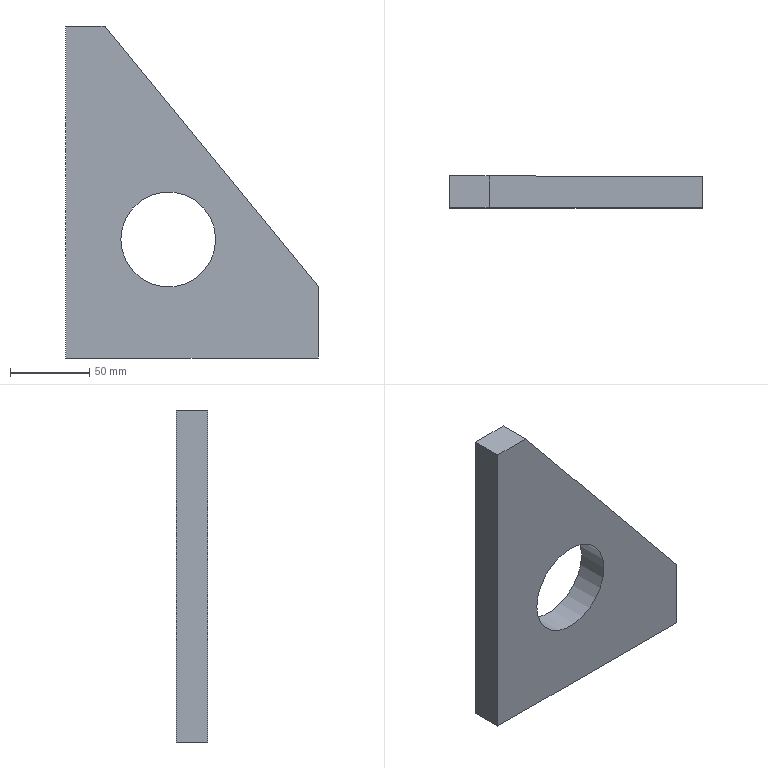Part | STEP file | Tube necking machine_id558_x_t | 1 solid | 8 faces | box 160 x 20 x 210 mm | volume 392701 mm3 | plane 7 | cylinder 1 | commonest cylinder face diameters 60 x1
STEP:
#1=CARTESIAN_POINT('',(0.,0.,0.));
#2=DIRECTION('',(0.,0.,1.));
#3=DIRECTION('',(1.,0.,0.));
#4=AXIS2_PLACEMENT_3D('',#1,#2,#3);
#5=CARTESIAN_POINT('',(387.5,115.,20.));
#6=VERTEX_POINT('',#5);
#7=CARTESIAN_POINT('',(387.5,115.,230.));
#8=VERTEX_POINT('',#7);
#9=CARTESIAN_POINT('',(387.5,115.,230.));
#10=DIRECTION('',(0.,0.,1.));
#11=VECTOR('',#10,1.);
#12=LINE('',#9,#11);
#13=CARTESIAN_POINT('',(387.5,95.,230.));
#14=DIRECTION('',(-1.,0.,0.));
#15=DIRECTION('',(0.,0.,1.));
#16=AXIS2_PLACEMENT_3D('',#13,#14,#15);
#17=PLANE('',#16);
#18=CARTESIAN_POINT('',(0.,20.));
#19=DIRECTION('',(1.,0.));
#20=VECTOR('',#19,1.);
#21=LINE('',#18,#20);
#22=(GEOMETRIC_REPRESENTATION_CONTEXT(2)PARAMETRIC_REPRESENTATION_CONTEXT()REPRESENTATION_CONTEXT('',''));
#23=DEFINITIONAL_REPRESENTATION('',(#21),#22);
#24=PCURVE('',#17,#23);
#25=CARTESIAN_POINT('',(452.5,115.,95.));
#26=DIRECTION('',(0.,1.,0.));
#27=DIRECTION('',(0.,0.,-1.));
#28=AXIS2_PLACEMENT_3D('',#25,#26,#27);
#29=PLANE('',#28);
#30=CARTESIAN_POINT('',(-135.,65.));
#31=DIRECTION('',(-1.,0.));
#32=VECTOR('',#31,1.);
#33=LINE('',#30,#32);
#34=(GEOMETRIC_REPRESENTATION_CONTEXT(2)PARAMETRIC_REPRESENTATION_CONTEXT()REPRESENTATION_CONTEXT('',''));
#35=DEFINITIONAL_REPRESENTATION('',(#33),#34);
#36=PCURVE('',#29,#35);
#37=SURFACE_CURVE('',#12,(#24,#36),.PCURVE_S1.);
#38=EDGE_CURVE('',#6,#8,#37,.T.);
#39=ORIENTED_EDGE('',*,*,#38,.F.);
#40=CARTESIAN_POINT('',(387.5,95.,20.));
#41=VERTEX_POINT('',#40);
#42=CARTESIAN_POINT('',(387.5,95.,20.));
#43=DIRECTION('',(0.,-1.,0.));
#44=VECTOR('',#43,1.);
#45=LINE('',#42,#44);
#46=CARTESIAN_POINT('',(-210.,0.));
#47=DIRECTION('',(0.,-1.));
#48=VECTOR('',#47,1.);
#49=LINE('',#46,#48);
#50=(GEOMETRIC_REPRESENTATION_CONTEXT(2)PARAMETRIC_REPRESENTATION_CONTEXT()REPRESENTATION_CONTEXT('',''));
#51=DEFINITIONAL_REPRESENTATION('',(#49),#50);
#52=PCURVE('',#17,#51);
#53=CARTESIAN_POINT('',(387.5,95.,20.));
#54=DIRECTION('',(0.,0.,-1.));
#55=DIRECTION('',(-1.,0.,0.));
#56=AXIS2_PLACEMENT_3D('',#53,#54,#55);
#57=PLANE('',#56);
#58=CARTESIAN_POINT('',(0.,0.));
#59=DIRECTION('',(0.,-1.));
#60=VECTOR('',#59,1.);
#61=LINE('',#58,#60);
#62=(GEOMETRIC_REPRESENTATION_CONTEXT(2)PARAMETRIC_REPRESENTATION_CONTEXT()REPRESENTATION_CONTEXT('',''));
#63=DEFINITIONAL_REPRESENTATION('',(#61),#62);
#64=PCURVE('',#57,#63);
#65=SURFACE_CURVE('',#45,(#52,#64),.PCURVE_S1.);
#66=EDGE_CURVE('',#6,#41,#65,.T.);
#67=ORIENTED_EDGE('',*,*,#66,.T.);
#68=CARTESIAN_POINT('',(387.5,95.,230.));
#69=VERTEX_POINT('',#68);
#70=CARTESIAN_POINT('',(387.5,95.,230.));
#71=DIRECTION('',(0.,0.,1.));
#72=VECTOR('',#71,1.);
#73=LINE('',#70,#72);
#74=CARTESIAN_POINT('',(0.,0.));
#75=DIRECTION('',(1.,0.));
#76=VECTOR('',#75,1.);
#77=LINE('',#74,#76);
#78=(GEOMETRIC_REPRESENTATION_CONTEXT(2)PARAMETRIC_REPRESENTATION_CONTEXT()REPRESENTATION_CONTEXT('',''));
#79=DEFINITIONAL_REPRESENTATION('',(#77),#78);
#80=PCURVE('',#17,#79);
#81=CARTESIAN_POINT('',(452.5,95.,95.));
#82=DIRECTION('',(0.,1.,0.));
#83=DIRECTION('',(0.,0.,-1.));
#84=AXIS2_PLACEMENT_3D('',#81,#82,#83);
#85=PLANE('',#84);
#86=CARTESIAN_POINT('',(-135.,65.));
#87=DIRECTION('',(-1.,0.));
#88=VECTOR('',#87,1.);
#89=LINE('',#86,#88);
#90=(GEOMETRIC_REPRESENTATION_CONTEXT(2)PARAMETRIC_REPRESENTATION_CONTEXT()REPRESENTATION_CONTEXT('',''));
#91=DEFINITIONAL_REPRESENTATION('',(#89),#90);
#92=PCURVE('',#85,#91);
#93=SURFACE_CURVE('',#73,(#80,#92),.PCURVE_S1.);
#94=EDGE_CURVE('',#41,#69,#93,.T.);
#95=ORIENTED_EDGE('',*,*,#94,.T.);
#96=CARTESIAN_POINT('',(387.5,95.,230.));
#97=DIRECTION('',(0.,-1.,0.));
#98=VECTOR('',#97,1.);
#99=LINE('',#96,#98);
#100=CARTESIAN_POINT('',(0.,0.));
#101=DIRECTION('',(0.,-1.));
#102=VECTOR('',#101,1.);
#103=LINE('',#100,#102);
#104=(GEOMETRIC_REPRESENTATION_CONTEXT(2)PARAMETRIC_REPRESENTATION_CONTEXT()REPRESENTATION_CONTEXT('',''));
#105=DEFINITIONAL_REPRESENTATION('',(#103),#104);
#106=PCURVE('',#17,#105);
#107=CARTESIAN_POINT('',(412.5,95.,230.));
#108=DIRECTION('',(0.,0.,1.));
#109=DIRECTION('',(1.,0.,0.));
#110=AXIS2_PLACEMENT_3D('',#107,#108,#109);
#111=PLANE('',#110);
#112=CARTESIAN_POINT('',(-25.,0.));
#113=DIRECTION('',(0.,-1.));
#114=VECTOR('',#113,1.);
#115=LINE('',#112,#114);
#116=(GEOMETRIC_REPRESENTATION_CONTEXT(2)PARAMETRIC_REPRESENTATION_CONTEXT()REPRESENTATION_CONTEXT('',''));
#117=DEFINITIONAL_REPRESENTATION('',(#115),#116);
#118=PCURVE('',#111,#117);
#119=SURFACE_CURVE('',#99,(#106,#118),.PCURVE_S1.);
#120=EDGE_CURVE('',#8,#69,#119,.T.);
#121=ORIENTED_EDGE('',*,*,#120,.F.);
#122=EDGE_LOOP('',(#39,#67,#95,#121));
#123=FACE_BOUND('',#122,.T.);
#124=ADVANCED_FACE('',(#123),#17,.T.);
#125=CARTESIAN_POINT('',(547.5,115.,20.));
#126=VERTEX_POINT('',#125);
#127=CARTESIAN_POINT('',(387.5,115.,20.));
#128=DIRECTION('',(-1.,0.,0.));
#129=VECTOR('',#128,1.);
#130=LINE('',#127,#129);
#131=CARTESIAN_POINT('',(0.,20.));
#132=DIRECTION('',(1.,0.));
#133=VECTOR('',#132,1.);
#134=LINE('',#131,#133);
#135=(GEOMETRIC_REPRESENTATION_CONTEXT(2)PARAMETRIC_REPRESENTATION_CONTEXT()REPRESENTATION_CONTEXT('',''));
#136=DEFINITIONAL_REPRESENTATION('',(#134),#135);
#137=PCURVE('',#57,#136);
#138=CARTESIAN_POINT('',(75.,65.));
#139=DIRECTION('',(0.,1.));
#140=VECTOR('',#139,1.);
#141=LINE('',#138,#140);
#142=(GEOMETRIC_REPRESENTATION_CONTEXT(2)PARAMETRIC_REPRESENTATION_CONTEXT()REPRESENTATION_CONTEXT('',''));
#143=DEFINITIONAL_REPRESENTATION('',(#141),#142);
#144=PCURVE('',#29,#143);
#145=SURFACE_CURVE('',#130,(#137,#144),.PCURVE_S1.);
#146=EDGE_CURVE('',#126,#6,#145,.T.);
#147=ORIENTED_EDGE('',*,*,#146,.F.);
#148=CARTESIAN_POINT('',(547.5,95.,20.));
#149=VERTEX_POINT('',#148);
#150=CARTESIAN_POINT('',(547.5,95.,20.));
#151=DIRECTION('',(0.,-1.,0.));
#152=VECTOR('',#151,1.);
#153=LINE('',#150,#152);
#154=CARTESIAN_POINT('',(-160.,0.));
#155=DIRECTION('',(0.,-1.));
#156=VECTOR('',#155,1.);
#157=LINE('',#154,#156);
#158=(GEOMETRIC_REPRESENTATION_CONTEXT(2)PARAMETRIC_REPRESENTATION_CONTEXT()REPRESENTATION_CONTEXT('',''));
#159=DEFINITIONAL_REPRESENTATION('',(#157),#158);
#160=PCURVE('',#57,#159);
#161=CARTESIAN_POINT('',(547.5,95.,20.));
#162=DIRECTION('',(1.,0.,0.));
#163=DIRECTION('',(0.,0.,-1.));
#164=AXIS2_PLACEMENT_3D('',#161,#162,#163);
#165=PLANE('',#164);
#166=CARTESIAN_POINT('',(0.,0.));
#167=DIRECTION('',(0.,-1.));
#168=VECTOR('',#167,1.);
#169=LINE('',#166,#168);
#170=(GEOMETRIC_REPRESENTATION_CONTEXT(2)PARAMETRIC_REPRESENTATION_CONTEXT()REPRESENTATION_CONTEXT('',''));
#171=DEFINITIONAL_REPRESENTATION('',(#169),#170);
#172=PCURVE('',#165,#171);
#173=SURFACE_CURVE('',#153,(#160,#172),.PCURVE_S1.);
#174=EDGE_CURVE('',#126,#149,#173,.T.);
#175=ORIENTED_EDGE('',*,*,#174,.T.);
#176=CARTESIAN_POINT('',(387.5,95.,20.));
#177=DIRECTION('',(-1.,0.,0.));
#178=VECTOR('',#177,1.);
#179=LINE('',#176,#178);
#180=CARTESIAN_POINT('',(0.,0.));
#181=DIRECTION('',(1.,0.));
#182=VECTOR('',#181,1.);
#183=LINE('',#180,#182);
#184=(GEOMETRIC_REPRESENTATION_CONTEXT(2)PARAMETRIC_REPRESENTATION_CONTEXT()REPRESENTATION_CONTEXT('',''));
#185=DEFINITIONAL_REPRESENTATION('',(#183),#184);
#186=PCURVE('',#57,#185);
#187=CARTESIAN_POINT('',(75.,65.));
#188=DIRECTION('',(0.,1.));
#189=VECTOR('',#188,1.);
#190=LINE('',#187,#189);
#191=(GEOMETRIC_REPRESENTATION_CONTEXT(2)PARAMETRIC_REPRESENTATION_CONTEXT()REPRESENTATION_CONTEXT('',''));
#192=DEFINITIONAL_REPRESENTATION('',(#190),#191);
#193=PCURVE('',#85,#192);
#194=SURFACE_CURVE('',#179,(#186,#193),.PCURVE_S1.);
#195=EDGE_CURVE('',#149,#41,#194,.T.);
#196=ORIENTED_EDGE('',*,*,#195,.T.);
#197=ORIENTED_EDGE('',*,*,#66,.F.);
#198=EDGE_LOOP('',(#147,#175,#196,#197));
#199=FACE_BOUND('',#198,.T.);
#200=ADVANCED_FACE('',(#199),#57,.T.);
#201=CARTESIAN_POINT('',(547.5,115.,65.));
#202=VERTEX_POINT('',#201);
#203=CARTESIAN_POINT('',(547.5,115.,20.));
#204=DIRECTION('',(0.,0.,-1.));
#205=VECTOR('',#204,1.);
#206=LINE('',#203,#205);
#207=CARTESIAN_POINT('',(0.,20.));
#208=DIRECTION('',(1.,0.));
#209=VECTOR('',#208,1.);
#210=LINE('',#207,#209);
#211=(GEOMETRIC_REPRESENTATION_CONTEXT(2)PARAMETRIC_REPRESENTATION_CONTEXT()REPRESENTATION_CONTEXT('',''));
#212=DEFINITIONAL_REPRESENTATION('',(#210),#211);
#213=PCURVE('',#165,#212);
#214=CARTESIAN_POINT('',(75.,-95.));
#215=DIRECTION('',(1.,0.));
#216=VECTOR('',#215,1.);
#217=LINE('',#214,#216);
#218=(GEOMETRIC_REPRESENTATION_CONTEXT(2)PARAMETRIC_REPRESENTATION_CONTEXT()REPRESENTATION_CONTEXT('',''));
#219=DEFINITIONAL_REPRESENTATION('',(#217),#218);
#220=PCURVE('',#29,#219);
#221=SURFACE_CURVE('',#206,(#213,#220),.PCURVE_S1.);
#222=EDGE_CURVE('',#202,#126,#221,.T.);
#223=ORIENTED_EDGE('',*,*,#222,.F.);
#224=CARTESIAN_POINT('',(547.5,95.,65.));
#225=VERTEX_POINT('',#224);
#226=CARTESIAN_POINT('',(547.5,95.,65.));
#227=DIRECTION('',(0.,-1.,0.));
#228=VECTOR('',#227,1.);
#229=LINE('',#226,#228);
#230=CARTESIAN_POINT('',(-45.,0.));
#231=DIRECTION('',(0.,-1.));
#232=VECTOR('',#231,1.);
#233=LINE('',#230,#232);
#234=(GEOMETRIC_REPRESENTATION_CONTEXT(2)PARAMETRIC_REPRESENTATION_CONTEXT()REPRESENTATION_CONTEXT('',''));
#235=DEFINITIONAL_REPRESENTATION('',(#233),#234);
#236=PCURVE('',#165,#235);
#237=CARTESIAN_POINT('',(547.5,95.,65.));
#238=DIRECTION('',(0.774,0.,0.6332));
#239=DIRECTION('',(0.6332,0.,-0.774));
#240=AXIS2_PLACEMENT_3D('',#237,#238,#239);
#241=PLANE('',#240);
#242=CARTESIAN_POINT('',(0.,0.));
#243=DIRECTION('',(0.,-1.));
#244=VECTOR('',#243,1.);
#245=LINE('',#242,#244);
#246=(GEOMETRIC_REPRESENTATION_CONTEXT(2)PARAMETRIC_REPRESENTATION_CONTEXT()REPRESENTATION_CONTEXT('',''));
#247=DEFINITIONAL_REPRESENTATION('',(#245),#246);
#248=PCURVE('',#241,#247);
#249=SURFACE_CURVE('',#229,(#236,#248),.PCURVE_S1.);
#250=EDGE_CURVE('',#202,#225,#249,.T.);
#251=ORIENTED_EDGE('',*,*,#250,.T.);
#252=CARTESIAN_POINT('',(547.5,95.,20.));
#253=DIRECTION('',(0.,0.,-1.));
#254=VECTOR('',#253,1.);
#255=LINE('',#252,#254);
#256=CARTESIAN_POINT('',(0.,0.));
#257=DIRECTION('',(1.,0.));
#258=VECTOR('',#257,1.);
#259=LINE('',#256,#258);
#260=(GEOMETRIC_REPRESENTATION_CONTEXT(2)PARAMETRIC_REPRESENTATION_CONTEXT()REPRESENTATION_CONTEXT('',''));
#261=DEFINITIONAL_REPRESENTATION('',(#259),#260);
#262=PCURVE('',#165,#261);
#263=CARTESIAN_POINT('',(75.,-95.));
#264=DIRECTION('',(1.,0.));
#265=VECTOR('',#264,1.);
#266=LINE('',#263,#265);
#267=(GEOMETRIC_REPRESENTATION_CONTEXT(2)PARAMETRIC_REPRESENTATION_CONTEXT()REPRESENTATION_CONTEXT('',''));
#268=DEFINITIONAL_REPRESENTATION('',(#266),#267);
#269=PCURVE('',#85,#268);
#270=SURFACE_CURVE('',#255,(#262,#269),.PCURVE_S1.);
#271=EDGE_CURVE('',#225,#149,#270,.T.);
#272=ORIENTED_EDGE('',*,*,#271,.T.);
#273=ORIENTED_EDGE('',*,*,#174,.F.);
#274=EDGE_LOOP('',(#223,#251,#272,#273));
#275=FACE_BOUND('',#274,.T.);
#276=ADVANCED_FACE('',(#275),#165,.T.);
#277=CARTESIAN_POINT('',(412.5,115.,230.));
#278=VERTEX_POINT('',#277);
#279=CARTESIAN_POINT('',(547.5,115.,65.));
#280=DIRECTION('',(0.6332,0.,-0.774));
#281=VECTOR('',#280,1.);
#282=LINE('',#279,#281);
#283=CARTESIAN_POINT('',(0.,20.));
#284=DIRECTION('',(1.,0.));
#285=VECTOR('',#284,1.);
#286=LINE('',#283,#285);
#287=(GEOMETRIC_REPRESENTATION_CONTEXT(2)PARAMETRIC_REPRESENTATION_CONTEXT()REPRESENTATION_CONTEXT('',''));
#288=DEFINITIONAL_REPRESENTATION('',(#286),#287);
#289=PCURVE('',#241,#288);
#290=CARTESIAN_POINT('',(30.,-95.));
#291=DIRECTION('',(0.774,-0.6332));
#292=VECTOR('',#291,1.);
#293=LINE('',#290,#292);
#294=(GEOMETRIC_REPRESENTATION_CONTEXT(2)PARAMETRIC_REPRESENTATION_CONTEXT()REPRESENTATION_CONTEXT('',''));
#295=DEFINITIONAL_REPRESENTATION('',(#293),#294);
#296=PCURVE('',#29,#295);
#297=SURFACE_CURVE('',#282,(#289,#296),.PCURVE_S1.);
#298=EDGE_CURVE('',#278,#202,#297,.T.);
#299=ORIENTED_EDGE('',*,*,#298,.F.);
#300=CARTESIAN_POINT('',(412.5,95.,230.));
#301=VERTEX_POINT('',#300);
#302=CARTESIAN_POINT('',(412.5,95.,230.));
#303=DIRECTION('',(0.,-1.,0.));
#304=VECTOR('',#303,1.);
#305=LINE('',#302,#304);
#306=CARTESIAN_POINT('',(-213.19,0.));
#307=DIRECTION('',(0.,-1.));
#308=VECTOR('',#307,1.);
#309=LINE('',#306,#308);
#310=(GEOMETRIC_REPRESENTATION_CONTEXT(2)PARAMETRIC_REPRESENTATION_CONTEXT()REPRESENTATION_CONTEXT('',''));
#311=DEFINITIONAL_REPRESENTATION('',(#309),#310);
#312=PCURVE('',#241,#311);
#313=CARTESIAN_POINT('',(0.,0.));
#314=DIRECTION('',(0.,-1.));
#315=VECTOR('',#314,1.);
#316=LINE('',#313,#315);
#317=(GEOMETRIC_REPRESENTATION_CONTEXT(2)PARAMETRIC_REPRESENTATION_CONTEXT()REPRESENTATION_CONTEXT('',''));
#318=DEFINITIONAL_REPRESENTATION('',(#316),#317);
#319=PCURVE('',#111,#318);
#320=SURFACE_CURVE('',#305,(#312,#319),.PCURVE_S1.);
#321=EDGE_CURVE('',#278,#301,#320,.T.);
#322=ORIENTED_EDGE('',*,*,#321,.T.);
#323=CARTESIAN_POINT('',(547.5,95.,65.));
#324=DIRECTION('',(0.6332,0.,-0.774));
#325=VECTOR('',#324,1.);
#326=LINE('',#323,#325);
#327=CARTESIAN_POINT('',(0.,0.));
#328=DIRECTION('',(1.,0.));
#329=VECTOR('',#328,1.);
#330=LINE('',#327,#329);
#331=(GEOMETRIC_REPRESENTATION_CONTEXT(2)PARAMETRIC_REPRESENTATION_CONTEXT()REPRESENTATION_CONTEXT('',''));
#332=DEFINITIONAL_REPRESENTATION('',(#330),#331);
#333=PCURVE('',#241,#332);
#334=CARTESIAN_POINT('',(30.,-95.));
#335=DIRECTION('',(0.774,-0.6332));
#336=VECTOR('',#335,1.);
#337=LINE('',#334,#336);
#338=(GEOMETRIC_REPRESENTATION_CONTEXT(2)PARAMETRIC_REPRESENTATION_CONTEXT()REPRESENTATION_CONTEXT('',''));
#339=DEFINITIONAL_REPRESENTATION('',(#337),#338);
#340=PCURVE('',#85,#339);
#341=SURFACE_CURVE('',#326,(#333,#340),.PCURVE_S1.);
#342=EDGE_CURVE('',#301,#225,#341,.T.);
#343=ORIENTED_EDGE('',*,*,#342,.T.);
#344=ORIENTED_EDGE('',*,*,#250,.F.);
#345=EDGE_LOOP('',(#299,#322,#343,#344));
#346=FACE_BOUND('',#345,.T.);
#347=ADVANCED_FACE('',(#346),#241,.T.);
#348=CARTESIAN_POINT('',(412.5,115.,230.));
#349=DIRECTION('',(1.,0.,0.));
#350=VECTOR('',#349,1.);
#351=LINE('',#348,#350);
#352=CARTESIAN_POINT('',(0.,20.));
#353=DIRECTION('',(1.,0.));
#354=VECTOR('',#353,1.);
#355=LINE('',#352,#354);
#356=(GEOMETRIC_REPRESENTATION_CONTEXT(2)PARAMETRIC_REPRESENTATION_CONTEXT()REPRESENTATION_CONTEXT('',''));
#357=DEFINITIONAL_REPRESENTATION('',(#355),#356);
#358=PCURVE('',#111,#357);
#359=CARTESIAN_POINT('',(-135.,40.));
#360=DIRECTION('',(0.,-1.));
#361=VECTOR('',#360,1.);
#362=LINE('',#359,#361);
#363=(GEOMETRIC_REPRESENTATION_CONTEXT(2)PARAMETRIC_REPRESENTATION_CONTEXT()REPRESENTATION_CONTEXT('',''));
#364=DEFINITIONAL_REPRESENTATION('',(#362),#363);
#365=PCURVE('',#29,#364);
#366=SURFACE_CURVE('',#351,(#358,#365),.PCURVE_S1.);
#367=EDGE_CURVE('',#8,#278,#366,.T.);
#368=ORIENTED_EDGE('',*,*,#367,.F.);
#369=ORIENTED_EDGE('',*,*,#120,.T.);
#370=CARTESIAN_POINT('',(412.5,95.,230.));
#371=DIRECTION('',(1.,0.,0.));
#372=VECTOR('',#371,1.);
#373=LINE('',#370,#372);
#374=CARTESIAN_POINT('',(0.,0.));
#375=DIRECTION('',(1.,0.));
#376=VECTOR('',#375,1.);
#377=LINE('',#374,#376);
#378=(GEOMETRIC_REPRESENTATION_CONTEXT(2)PARAMETRIC_REPRESENTATION_CONTEXT()REPRESENTATION_CONTEXT('',''));
#379=DEFINITIONAL_REPRESENTATION('',(#377),#378);
#380=PCURVE('',#111,#379);
#381=CARTESIAN_POINT('',(-135.,40.));
#382=DIRECTION('',(0.,-1.));
#383=VECTOR('',#382,1.);
#384=LINE('',#381,#383);
#385=(GEOMETRIC_REPRESENTATION_CONTEXT(2)PARAMETRIC_REPRESENTATION_CONTEXT()REPRESENTATION_CONTEXT('',''));
#386=DEFINITIONAL_REPRESENTATION('',(#384),#385);
#387=PCURVE('',#85,#386);
#388=SURFACE_CURVE('',#373,(#380,#387),.PCURVE_S1.);
#389=EDGE_CURVE('',#69,#301,#388,.T.);
#390=ORIENTED_EDGE('',*,*,#389,.T.);
#391=ORIENTED_EDGE('',*,*,#321,.F.);
#392=EDGE_LOOP('',(#368,#369,#390,#391));
#393=FACE_BOUND('',#392,.T.);
#394=ADVANCED_FACE('',(#393),#111,.T.);
#395=CARTESIAN_POINT('',(482.5,95.,95.));
#396=VERTEX_POINT('',#395);
#397=CARTESIAN_POINT('',(452.5,95.,95.));
#398=DIRECTION('',(0.,1.,0.));
#399=DIRECTION('',(1.,0.,0.));
#400=AXIS2_PLACEMENT_3D('',#397,#398,#399);
#401=CIRCLE('',#400,30.);
#402=CARTESIAN_POINT('',(452.5,95.,95.));
#403=DIRECTION('',(0.,1.,0.));
#404=DIRECTION('',(0.,0.,-1.));
#405=AXIS2_PLACEMENT_3D('',#402,#403,#404);
#406=CYLINDRICAL_SURFACE('',#405,30.);
#407=CARTESIAN_POINT('',(4.712,0.));
#408=DIRECTION('',(1.,0.));
#409=VECTOR('',#408,1.);
#410=LINE('',#407,#409);
#411=(GEOMETRIC_REPRESENTATION_CONTEXT(2)PARAMETRIC_REPRESENTATION_CONTEXT()REPRESENTATION_CONTEXT('',''));
#412=DEFINITIONAL_REPRESENTATION('',(#410),#411);
#413=PCURVE('',#406,#412);
#414=CARTESIAN_POINT('',(0.,0.));
#415=DIRECTION('',(0.,-1.));
#416=AXIS2_PLACEMENT_2D('',#414,#415);
#417=CIRCLE('',#416,30.);
#418=(GEOMETRIC_REPRESENTATION_CONTEXT(2)PARAMETRIC_REPRESENTATION_CONTEXT()REPRESENTATION_CONTEXT('',''));
#419=DEFINITIONAL_REPRESENTATION('',(#417),#418);
#420=PCURVE('',#85,#419);
#421=SURFACE_CURVE('',#401,(#413,#420),.PCURVE_S1.);
#422=EDGE_CURVE('',#396,#396,#421,.T.);
#423=ORIENTED_EDGE('',*,*,#422,.T.);
#424=CARTESIAN_POINT('',(482.5,115.,95.));
#425=VERTEX_POINT('',#424);
#426=CARTESIAN_POINT('',(482.5,95.,95.));
#427=CARTESIAN_POINT('',(482.5,115.,95.));
#428=B_SPLINE_CURVE_WITH_KNOTS('',1,(#426,#427),.UNSPECIFIED.,.F.,.F.,(2,2),(0.,20.),.PIECEWISE_BEZIER_KNOTS.);
#429=CARTESIAN_POINT('',(10.996,0.));
#430=DIRECTION('',(0.,1.));
#431=VECTOR('',#430,1.);
#432=LINE('',#429,#431);
#433=(GEOMETRIC_REPRESENTATION_CONTEXT(2)PARAMETRIC_REPRESENTATION_CONTEXT()REPRESENTATION_CONTEXT('',''));
#434=DEFINITIONAL_REPRESENTATION('',(#432),#433);
#435=PCURVE('',#406,#434);
#436=CARTESIAN_POINT('',(4.712,0.));
#437=DIRECTION('',(0.,1.));
#438=VECTOR('',#437,1.);
#439=LINE('',#436,#438);
#440=(GEOMETRIC_REPRESENTATION_CONTEXT(2)PARAMETRIC_REPRESENTATION_CONTEXT()REPRESENTATION_CONTEXT('',''));
#441=DEFINITIONAL_REPRESENTATION('',(#439),#440);
#442=PCURVE('',#406,#441);
#443=SEAM_CURVE('',#428,(#435,#442),.PCURVE_S1.);
#444=EDGE_CURVE('',#396,#425,#443,.T.);
#445=ORIENTED_EDGE('',*,*,#444,.T.);
#446=CARTESIAN_POINT('',(452.5,115.,95.));
#447=DIRECTION('',(0.,1.,0.));
#448=DIRECTION('',(1.,0.,0.));
#449=AXIS2_PLACEMENT_3D('',#446,#447,#448);
#450=CIRCLE('',#449,30.);
#451=CARTESIAN_POINT('',(4.712,20.));
#452=DIRECTION('',(1.,0.));
#453=VECTOR('',#452,1.);
#454=LINE('',#451,#453);
#455=(GEOMETRIC_REPRESENTATION_CONTEXT(2)PARAMETRIC_REPRESENTATION_CONTEXT()REPRESENTATION_CONTEXT('',''));
#456=DEFINITIONAL_REPRESENTATION('',(#454),#455);
#457=PCURVE('',#406,#456);
#458=CARTESIAN_POINT('',(0.,0.));
#459=DIRECTION('',(0.,-1.));
#460=AXIS2_PLACEMENT_2D('',#458,#459);
#461=CIRCLE('',#460,30.);
#462=(GEOMETRIC_REPRESENTATION_CONTEXT(2)PARAMETRIC_REPRESENTATION_CONTEXT()REPRESENTATION_CONTEXT('',''));
#463=DEFINITIONAL_REPRESENTATION('',(#461),#462);
#464=PCURVE('',#29,#463);
#465=SURFACE_CURVE('',#450,(#457,#464),.PCURVE_S1.);
#466=EDGE_CURVE('',#425,#425,#465,.T.);
#467=ORIENTED_EDGE('',*,*,#466,.F.);
#468=ORIENTED_EDGE('',*,*,#444,.F.);
#469=EDGE_LOOP('',(#423,#445,#467,#468));
#470=FACE_BOUND('',#469,.F.);
#471=ADVANCED_FACE('',(#470),#406,.F.);
#472=ORIENTED_EDGE('',*,*,#94,.F.);
#473=ORIENTED_EDGE('',*,*,#195,.F.);
#474=ORIENTED_EDGE('',*,*,#271,.F.);
#475=ORIENTED_EDGE('',*,*,#342,.F.);
#476=ORIENTED_EDGE('',*,*,#389,.F.);
#477=EDGE_LOOP('',(#472,#473,#474,#475,#476));
#478=FACE_BOUND('',#477,.T.);
#479=ORIENTED_EDGE('',*,*,#422,.T.);
#480=EDGE_LOOP('',(#479));
#481=FACE_BOUND('',#480,.T.);
#482=ADVANCED_FACE('',(#478,#481),#85,.F.);
#483=ORIENTED_EDGE('',*,*,#38,.T.);
#484=ORIENTED_EDGE('',*,*,#367,.T.);
#485=ORIENTED_EDGE('',*,*,#298,.T.);
#486=ORIENTED_EDGE('',*,*,#222,.T.);
#487=ORIENTED_EDGE('',*,*,#146,.T.);
#488=EDGE_LOOP('',(#483,#484,#485,#486,#487));
#489=FACE_BOUND('',#488,.T.);
#490=ORIENTED_EDGE('',*,*,#466,.F.);
#491=EDGE_LOOP('',(#490));
#492=FACE_BOUND('',#491,.T.);
#493=ADVANCED_FACE('',(#489,#492),#29,.T.);
#494=CLOSED_SHELL('',(#124,#200,#276,#347,#394,#471,#482,#493));
#495=MANIFOLD_SOLID_BREP('',#494);
#496=(LENGTH_UNIT()NAMED_UNIT(*)SI_UNIT(.MILLI.,.METRE.));
#497=UNCERTAINTY_MEASURE_WITH_UNIT(LENGTH_MEASURE(0.000001),#496,'','');
#498=(NAMED_UNIT(*)PLANE_ANGLE_UNIT()SI_UNIT($,.RADIAN.));
#499=(NAMED_UNIT(*)SI_UNIT($,.STERADIAN.)SOLID_ANGLE_UNIT());
#500=(GEOMETRIC_REPRESENTATION_CONTEXT(3)GLOBAL_UNCERTAINTY_ASSIGNED_CONTEXT((#497))GLOBAL_UNIT_ASSIGNED_CONTEXT((#496,#498,#499))REPRESENTATION_CONTEXT('',''));
#501=ADVANCED_BREP_SHAPE_REPRESENTATION('',(#4,#495),#500);